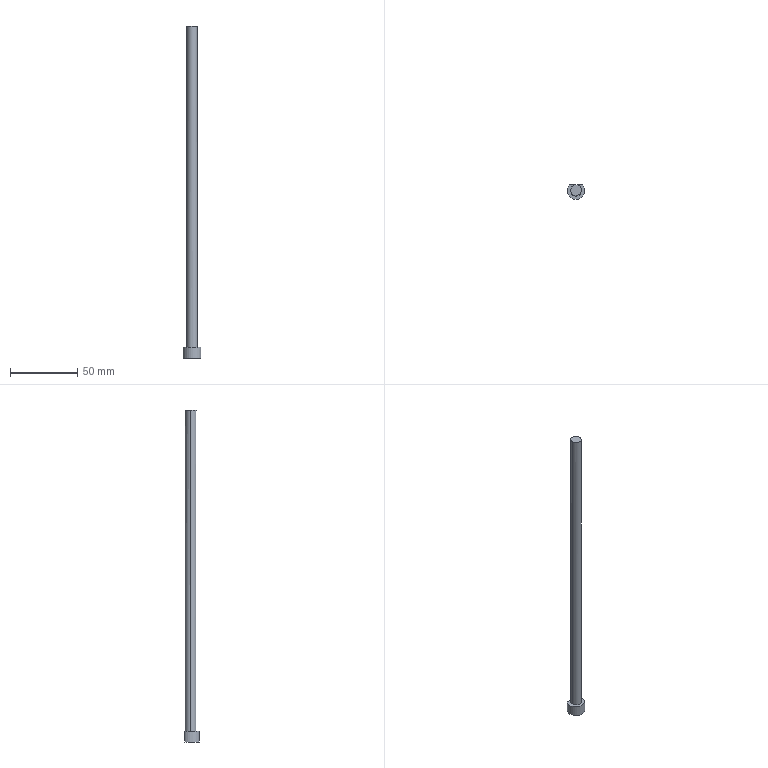Part | Creo | 1 solid | 7 faces | box 13 x 11 x 247.048 mm | volume 12974 mm3 | plane 4 | cylinder 3 | commonest cylinder face diameters 8 x2 13 x1
STEP:
#1=CARTESIAN_POINT('',(0.,0.,0.));
#2=DIRECTION('',(0.,0.,1.));
#3=DIRECTION('',(1.,0.,0.));
#4=AXIS2_PLACEMENT_3D('',#1,#2,#3);
#5=CARTESIAN_POINT('',(-83.574,-2.902,-330.441));
#6=VERTEX_POINT('',#5);
#7=CARTESIAN_POINT('',(-92.955,-2.902,-330.441));
#8=VERTEX_POINT('',#7);
#9=CARTESIAN_POINT('',(-83.574,-2.902,-330.441));
#10=DIRECTION('',(-1.,0.,0.));
#11=VECTOR('',#10,9.381);
#12=LINE('',#9,#11);
#13=EDGE_CURVE('',#6,#8,#12,.T.);
#14=ORIENTED_EDGE('',*,*,#13,.F.);
#15=CARTESIAN_POINT('',(-88.264,-7.402,-330.441));
#16=DIRECTION('',(0.,0.,-1.));
#17=DIRECTION('',(0.7216,0.6923,0.));
#18=AXIS2_PLACEMENT_3D('',#15,#16,#17);
#19=CIRCLE('',#18,6.5);
#20=EDGE_CURVE('',#6,#8,#19,.T.);
#21=ORIENTED_EDGE('',*,*,#20,.T.);
#22=EDGE_LOOP('',(#14,#21));
#23=FACE_OUTER_BOUND('',#22,.F.);
#24=CARTESIAN_POINT('',(-92.264,-7.402,-330.441));
#25=VERTEX_POINT('',#24);
#26=CARTESIAN_POINT('',(-84.264,-7.402,-330.441));
#27=VERTEX_POINT('',#26);
#28=CARTESIAN_POINT('',(-88.264,-7.402,-330.441));
#29=DIRECTION('',(0.,0.,-1.));
#30=DIRECTION('',(-1.,0.,0.));
#31=AXIS2_PLACEMENT_3D('',#28,#29,#30);
#32=CIRCLE('',#31,4.);
#33=EDGE_CURVE('',#25,#27,#32,.T.);
#34=ORIENTED_EDGE('',*,*,#33,.F.);
#35=CARTESIAN_POINT('',(-88.264,-7.402,-330.441));
#36=DIRECTION('',(0.,0.,-1.));
#37=DIRECTION('',(1.,0.,0.));
#38=AXIS2_PLACEMENT_3D('',#35,#36,#37);
#39=CIRCLE('',#38,4.);
#40=EDGE_CURVE('',#27,#25,#39,.T.);
#41=ORIENTED_EDGE('',*,*,#40,.F.);
#42=EDGE_LOOP('',(#34,#41));
#43=FACE_BOUND('',#42,.F.);
#44=CARTESIAN_POINT('',(-88.264,-7.402,-330.441));
#45=DIRECTION('',(0.,0.,-1.));
#46=DIRECTION('',(-1.,0.,0.));
#47=AXIS2_PLACEMENT_3D('',#44,#45,#46);
#48=PLANE('',#47);
#49=ADVANCED_FACE('',(#23,#43),#48,.F.);
#50=CARTESIAN_POINT('',(-84.264,-7.402,-91.404));
#51=VERTEX_POINT('',#50);
#52=CARTESIAN_POINT('',(-92.264,-7.401,-91.394));
#53=VERTEX_POINT('',#52);
#54=CARTESIAN_POINT('',(-84.264,-7.402,-91.404));
#55=CARTESIAN_POINT('',(-84.264,-7.009,-91.404));
#56=CARTESIAN_POINT('',(-84.375,-6.259,-91.404));
#57=CARTESIAN_POINT('',(-84.857,-5.203,-91.404));
#58=CARTESIAN_POINT('',(-85.614,-4.334,-91.403));
#59=CARTESIAN_POINT('',(-86.583,-3.713,-91.401));
#60=CARTESIAN_POINT('',(-87.687,-3.389,-91.4));
#61=CARTESIAN_POINT('',(-88.837,-3.389,-91.398));
#62=CARTESIAN_POINT('',(-89.941,-3.711,-91.397));
#63=CARTESIAN_POINT('',(-90.911,-4.331,-91.396));
#64=CARTESIAN_POINT('',(-91.669,-5.199,-91.395));
#65=CARTESIAN_POINT('',(-92.152,-6.253,-91.394));
#66=CARTESIAN_POINT('',(-92.264,-7.008,-91.394));
#67=CARTESIAN_POINT('',(-92.264,-7.401,-91.394));
#68=B_SPLINE_CURVE_WITH_KNOTS('',3,(#54,#55,#56,#57,#58,#59,#60,#61,#62,#63,#64,#65,#66,#67),.UNSPECIFIED.,.F.,.F.,(4,1,1,1,1,1,1,1,1,1,1,4),(0.,0.09091,0.1818,0.2727,0.3636,0.4545,0.5455,0.6364,0.7273,0.8182,0.9091,1.),.UNSPECIFIED.);
#69=EDGE_CURVE('',#51,#53,#68,.T.);
#70=ORIENTED_EDGE('',*,*,#69,.T.);
#71=CARTESIAN_POINT('',(-92.264,-7.402,-330.441));
#72=DIRECTION('',(0.000000004,0.000007078,1.));
#73=VECTOR('',#72,239.048);
#74=LINE('',#71,#73);
#75=EDGE_CURVE('',#25,#53,#74,.T.);
#76=ORIENTED_EDGE('',*,*,#75,.F.);
#77=ORIENTED_EDGE('',*,*,#33,.T.);
#78=CARTESIAN_POINT('',(-84.264,-7.402,-330.441));
#79=DIRECTION('',(0.,0.,1.));
#80=VECTOR('',#79,239.037);
#81=LINE('',#78,#80);
#82=EDGE_CURVE('',#27,#51,#81,.T.);
#83=ORIENTED_EDGE('',*,*,#82,.T.);
#84=EDGE_LOOP('',(#70,#76,#77,#83));
#85=FACE_OUTER_BOUND('',#84,.F.);
#86=CARTESIAN_POINT('',(-88.264,-7.402,-653.441));
#87=DIRECTION('',(0.,0.,1.));
#88=DIRECTION('',(1.,0.,0.));
#89=AXIS2_PLACEMENT_3D('',#86,#87,#88);
#90=CYLINDRICAL_SURFACE('',#89,4.);
#91=ADVANCED_FACE('',(#85),#90,.T.);
#92=CARTESIAN_POINT('',(-92.264,-7.401,-91.394));
#93=CARTESIAN_POINT('',(-92.264,-7.796,-91.394));
#94=CARTESIAN_POINT('',(-92.154,-8.544,-91.394));
#95=CARTESIAN_POINT('',(-91.672,-9.6,-91.395));
#96=CARTESIAN_POINT('',(-90.923,-10.461,-91.396));
#97=CARTESIAN_POINT('',(-89.963,-11.084,-91.397));
#98=CARTESIAN_POINT('',(-88.855,-11.414,-91.398));
#99=CARTESIAN_POINT('',(-87.706,-11.418,-91.4));
#100=CARTESIAN_POINT('',(-86.597,-11.099,-91.401));
#101=CARTESIAN_POINT('',(-85.627,-10.481,-91.403));
#102=CARTESIAN_POINT('',(-84.864,-9.615,-91.404));
#103=CARTESIAN_POINT('',(-84.375,-8.548,-91.404));
#104=CARTESIAN_POINT('',(-84.264,-7.796,-91.404));
#105=CARTESIAN_POINT('',(-84.264,-7.402,-91.404));
#106=B_SPLINE_CURVE_WITH_KNOTS('',3,(#92,#93,#94,#95,#96,#97,#98,#99,#100,#101,#102,#103,#104,#105),.UNSPECIFIED.,.F.,.F.,(4,1,1,1,1,1,1,1,1,1,1,4),(0.,0.09091,0.1818,0.2727,0.3636,0.4545,0.5455,0.6364,0.7273,0.8182,0.9091,1.),.UNSPECIFIED.);
#107=EDGE_CURVE('',#53,#51,#106,.T.);
#108=ORIENTED_EDGE('',*,*,#107,.F.);
#109=ORIENTED_EDGE('',*,*,#69,.F.);
#110=EDGE_LOOP('',(#108,#109));
#111=FACE_OUTER_BOUND('',#110,.F.);
#112=CARTESIAN_POINT('',(248.993,54.022,-91.842));
#113=DIRECTION('',(-0.001312,0.000001665,-1.));
#114=DIRECTION('',(-1.,0.,0.001312));
#115=AXIS2_PLACEMENT_3D('',#112,#113,#114);
#116=PLANE('',#115);
#117=ADVANCED_FACE('',(#111),#116,.F.);
#118=ORIENTED_EDGE('',*,*,#107,.T.);
#119=ORIENTED_EDGE('',*,*,#82,.F.);
#120=ORIENTED_EDGE('',*,*,#40,.T.);
#121=ORIENTED_EDGE('',*,*,#75,.T.);
#122=EDGE_LOOP('',(#118,#119,#120,#121));
#123=FACE_OUTER_BOUND('',#122,.F.);
#124=CARTESIAN_POINT('',(-88.264,-7.402,-653.441));
#125=DIRECTION('',(0.,0.,1.));
#126=DIRECTION('',(1.,0.,0.));
#127=AXIS2_PLACEMENT_3D('',#124,#125,#126);
#128=CYLINDRICAL_SURFACE('',#127,4.);
#129=ADVANCED_FACE('',(#123),#128,.T.);
#130=CARTESIAN_POINT('',(-92.955,-2.902,-338.441));
#131=VERTEX_POINT('',#130);
#132=CARTESIAN_POINT('',(-92.955,-2.902,-330.441));
#133=DIRECTION('',(0.,0.,-1.));
#134=VECTOR('',#133,8.);
#135=LINE('',#132,#134);
#136=EDGE_CURVE('',#8,#131,#135,.T.);
#137=ORIENTED_EDGE('',*,*,#136,.T.);
#138=CARTESIAN_POINT('',(-83.574,-2.902,-338.441));
#139=VERTEX_POINT('',#138);
#140=CARTESIAN_POINT('',(-83.574,-2.902,-338.441));
#141=DIRECTION('',(-1.,0.,0.));
#142=VECTOR('',#141,9.381);
#143=LINE('',#140,#142);
#144=EDGE_CURVE('',#139,#131,#143,.T.);
#145=ORIENTED_EDGE('',*,*,#144,.F.);
#146=CARTESIAN_POINT('',(-83.574,-2.902,-338.441));
#147=DIRECTION('',(0.,0.,1.));
#148=VECTOR('',#147,8.);
#149=LINE('',#146,#148);
#150=EDGE_CURVE('',#139,#6,#149,.T.);
#151=ORIENTED_EDGE('',*,*,#150,.T.);
#152=ORIENTED_EDGE('',*,*,#13,.T.);
#153=EDGE_LOOP('',(#137,#145,#151,#152));
#154=FACE_OUTER_BOUND('',#153,.F.);
#155=CARTESIAN_POINT('',(-88.264,-2.902,-338.441));
#156=DIRECTION('',(0.,1.,0.));
#157=DIRECTION('',(0.,0.,1.));
#158=AXIS2_PLACEMENT_3D('',#155,#156,#157);
#159=PLANE('',#158);
#160=ADVANCED_FACE('',(#154),#159,.T.);
#161=CARTESIAN_POINT('',(-88.264,-7.402,-338.441));
#162=DIRECTION('',(0.,0.,1.));
#163=DIRECTION('',(-0.7216,0.6923,0.));
#164=AXIS2_PLACEMENT_3D('',#161,#162,#163);
#165=CIRCLE('',#164,6.5);
#166=EDGE_CURVE('',#131,#139,#165,.T.);
#167=ORIENTED_EDGE('',*,*,#166,.F.);
#168=ORIENTED_EDGE('',*,*,#136,.F.);
#169=ORIENTED_EDGE('',*,*,#20,.F.);
#170=ORIENTED_EDGE('',*,*,#150,.F.);
#171=EDGE_LOOP('',(#167,#168,#169,#170));
#172=FACE_OUTER_BOUND('',#171,.F.);
#173=CARTESIAN_POINT('',(-88.264,-7.402,-330.441));
#174=DIRECTION('',(0.,0.,-1.));
#175=DIRECTION('',(-1.,0.,0.));
#176=AXIS2_PLACEMENT_3D('',#173,#174,#175);
#177=CYLINDRICAL_SURFACE('',#176,6.5);
#178=ADVANCED_FACE('',(#172),#177,.T.);
#179=ORIENTED_EDGE('',*,*,#166,.T.);
#180=ORIENTED_EDGE('',*,*,#144,.T.);
#181=EDGE_LOOP('',(#179,#180));
#182=FACE_OUTER_BOUND('',#181,.F.);
#183=CARTESIAN_POINT('',(-88.264,-7.402,-338.441));
#184=DIRECTION('',(0.,0.,-1.));
#185=DIRECTION('',(-1.,0.,0.));
#186=AXIS2_PLACEMENT_3D('',#183,#184,#185);
#187=PLANE('',#186);
#188=ADVANCED_FACE('',(#182),#187,.T.);
#189=CLOSED_SHELL('',(#49,#91,#117,#129,#160,#178,#188));
#190=MANIFOLD_SOLID_BREP('',#189);
#191=(LENGTH_UNIT()NAMED_UNIT(*)SI_UNIT(.MILLI.,.METRE.));
#192=UNCERTAINTY_MEASURE_WITH_UNIT(LENGTH_MEASURE(0.02476),#191,'','');
#193=(NAMED_UNIT(*)PLANE_ANGLE_UNIT()SI_UNIT($,.RADIAN.));
#194=PLANE_ANGLE_MEASURE_WITH_UNIT(PLANE_ANGLE_MEASURE(0.01745),#193);
#195=(CONVERSION_BASED_UNIT('DEGREE',#194)NAMED_UNIT(*)PLANE_ANGLE_UNIT());
#196=(NAMED_UNIT(*)SI_UNIT($,.STERADIAN.)SOLID_ANGLE_UNIT());
#197=(GEOMETRIC_REPRESENTATION_CONTEXT(3)GLOBAL_UNCERTAINTY_ASSIGNED_CONTEXT((#192))GLOBAL_UNIT_ASSIGNED_CONTEXT((#191,#195,#196))REPRESENTATION_CONTEXT('',''));
#198=ADVANCED_BREP_SHAPE_REPRESENTATION('',(#4,#190),#197);